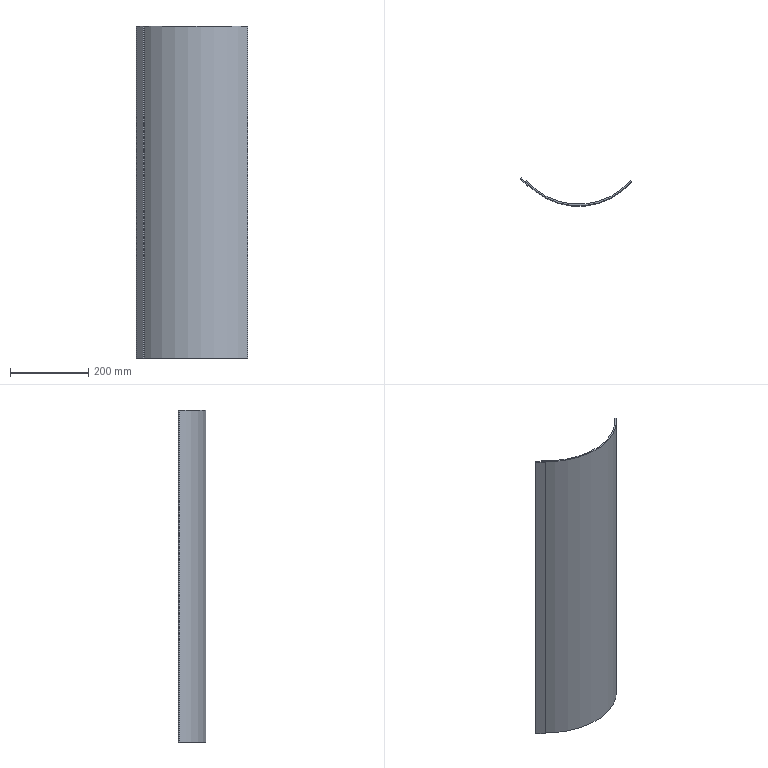Part | SolidWorks | features ExtruThin 1, ICE 1 | 2 solids | 12 faces | box 284.209 x 71.481 x 850 mm | volume 1096694 mm3 | plane 10 | cylinder 2 | commonest cylinder face diameters 354 x1 362 x1
STEP:
#1=CARTESIAN_POINT('',(-135.817,-119.644,-425.));
#2=VERTEX_POINT('',#1);
#3=CARTESIAN_POINT('',(135.817,-119.644,-425.));
#4=VERTEX_POINT('',#3);
#5=CARTESIAN_POINT('',(0.,0.,-425.));
#6=DIRECTION('',(0.,0.,1.));
#7=DIRECTION('',(1.,0.,0.));
#8=AXIS2_PLACEMENT_3D('',#5,#6,#7);
#9=CIRCLE('',#8,181.);
#10=EDGE_CURVE('',#2,#4,#9,.T.);
#11=ORIENTED_EDGE('',*,*,#10,.T.);
#12=CARTESIAN_POINT('',(135.817,-119.644,425.));
#13=VERTEX_POINT('',#12);
#14=CARTESIAN_POINT('',(135.817,-119.644,425.));
#15=DIRECTION('',(0.,0.,-1.));
#16=VECTOR('',#15,1000.);
#17=LINE('',#14,#16);
#18=EDGE_CURVE('',#13,#4,#17,.T.);
#19=ORIENTED_EDGE('',*,*,#18,.F.);
#20=CARTESIAN_POINT('',(-135.817,-119.644,425.));
#21=VERTEX_POINT('',#20);
#22=CARTESIAN_POINT('',(0.,0.,425.));
#23=DIRECTION('',(0.,0.,1.));
#24=DIRECTION('',(1.,0.,0.));
#25=AXIS2_PLACEMENT_3D('',#22,#23,#24);
#26=CIRCLE('',#25,181.);
#27=EDGE_CURVE('',#21,#13,#26,.T.);
#28=ORIENTED_EDGE('',*,*,#27,.F.);
#29=CARTESIAN_POINT('',(-135.817,-119.644,425.));
#30=DIRECTION('',(0.,0.,-1.));
#31=VECTOR('',#30,1000.);
#32=LINE('',#29,#31);
#33=EDGE_CURVE('',#21,#2,#32,.T.);
#34=ORIENTED_EDGE('',*,*,#33,.T.);
#35=EDGE_LOOP('',(#11,#19,#28,#34));
#36=FACE_OUTER_BOUND('',#35,.T.);
#37=CARTESIAN_POINT('',(0.,0.,425.));
#38=DIRECTION('',(0.,0.,-1.));
#39=DIRECTION('',(-1.,0.,0.));
#40=AXIS2_PLACEMENT_3D('',#37,#38,#39);
#41=CYLINDRICAL_SURFACE('',#40,181.);
#42=ADVANCED_FACE('',(#36),#41,.T.);
#43=CARTESIAN_POINT('',(132.816,-117.,-425.));
#44=VERTEX_POINT('',#43);
#45=CARTESIAN_POINT('',(132.816,-117.,-425.));
#46=DIRECTION('',(0.7504,-0.661,0.));
#47=VECTOR('',#46,1000.);
#48=LINE('',#45,#47);
#49=EDGE_CURVE('',#44,#4,#48,.T.);
#50=ORIENTED_EDGE('',*,*,#49,.F.);
#51=CARTESIAN_POINT('',(132.816,-117.,425.));
#52=VERTEX_POINT('',#51);
#53=CARTESIAN_POINT('',(132.816,-117.,425.));
#54=DIRECTION('',(0.,0.,-1.));
#55=VECTOR('',#54,1000.);
#56=LINE('',#53,#55);
#57=EDGE_CURVE('',#52,#44,#56,.T.);
#58=ORIENTED_EDGE('',*,*,#57,.F.);
#59=CARTESIAN_POINT('',(132.816,-117.,425.));
#60=DIRECTION('',(0.7504,-0.661,0.));
#61=VECTOR('',#60,1000.);
#62=LINE('',#59,#61);
#63=EDGE_CURVE('',#52,#13,#62,.T.);
#64=ORIENTED_EDGE('',*,*,#63,.T.);
#65=ORIENTED_EDGE('',*,*,#18,.T.);
#66=EDGE_LOOP('',(#50,#58,#64,#65));
#67=FACE_OUTER_BOUND('',#66,.T.);
#68=CARTESIAN_POINT('',(132.816,-117.,425.));
#69=DIRECTION('',(0.661,0.7504,0.));
#70=DIRECTION('',(-0.7504,0.661,0.));
#71=AXIS2_PLACEMENT_3D('',#68,#69,#70);
#72=PLANE('',#71);
#73=ADVANCED_FACE('',(#67),#72,.T.);
#74=CARTESIAN_POINT('',(-132.816,-117.,-425.));
#75=VERTEX_POINT('',#74);
#76=CARTESIAN_POINT('',(0.,0.,-425.));
#77=DIRECTION('',(0.,0.,1.));
#78=DIRECTION('',(1.,0.,0.));
#79=AXIS2_PLACEMENT_3D('',#76,#77,#78);
#80=CIRCLE('',#79,177.);
#81=EDGE_CURVE('',#75,#44,#80,.T.);
#82=ORIENTED_EDGE('',*,*,#81,.F.);
#83=CARTESIAN_POINT('',(-132.816,-117.,425.));
#84=VERTEX_POINT('',#83);
#85=CARTESIAN_POINT('',(-132.816,-117.,425.));
#86=DIRECTION('',(0.,0.,-1.));
#87=VECTOR('',#86,1000.);
#88=LINE('',#85,#87);
#89=EDGE_CURVE('',#84,#75,#88,.T.);
#90=ORIENTED_EDGE('',*,*,#89,.F.);
#91=CARTESIAN_POINT('',(0.,0.,425.));
#92=DIRECTION('',(0.,0.,1.));
#93=DIRECTION('',(1.,0.,0.));
#94=AXIS2_PLACEMENT_3D('',#91,#92,#93);
#95=CIRCLE('',#94,177.);
#96=EDGE_CURVE('',#84,#52,#95,.T.);
#97=ORIENTED_EDGE('',*,*,#96,.T.);
#98=ORIENTED_EDGE('',*,*,#57,.T.);
#99=EDGE_LOOP('',(#82,#90,#97,#98));
#100=FACE_OUTER_BOUND('',#99,.T.);
#101=CARTESIAN_POINT('',(0.,0.,425.));
#102=DIRECTION('',(0.,0.,-1.));
#103=DIRECTION('',(-1.,0.,0.));
#104=AXIS2_PLACEMENT_3D('',#101,#102,#103);
#105=CYLINDRICAL_SURFACE('',#104,177.);
#106=ADVANCED_FACE('',(#100),#105,.F.);
#107=CARTESIAN_POINT('',(-135.817,-119.644,-425.));
#108=DIRECTION('',(0.7504,0.661,0.));
#109=VECTOR('',#108,1000.);
#110=LINE('',#107,#109);
#111=EDGE_CURVE('',#2,#75,#110,.T.);
#112=ORIENTED_EDGE('',*,*,#111,.F.);
#113=ORIENTED_EDGE('',*,*,#33,.F.);
#114=CARTESIAN_POINT('',(-135.817,-119.644,425.));
#115=DIRECTION('',(0.7504,0.661,0.));
#116=VECTOR('',#115,1000.);
#117=LINE('',#114,#116);
#118=EDGE_CURVE('',#21,#84,#117,.T.);
#119=ORIENTED_EDGE('',*,*,#118,.T.);
#120=ORIENTED_EDGE('',*,*,#89,.T.);
#121=EDGE_LOOP('',(#112,#113,#119,#120));
#122=FACE_OUTER_BOUND('',#121,.T.);
#123=CARTESIAN_POINT('',(-135.817,-119.644,425.));
#124=DIRECTION('',(-0.661,0.7504,0.));
#125=DIRECTION('',(-0.7504,-0.661,0.));
#126=AXIS2_PLACEMENT_3D('',#123,#124,#125);
#127=PLANE('',#126);
#128=ADVANCED_FACE('',(#122),#127,.T.);
#129=ORIENTED_EDGE('',*,*,#27,.T.);
#130=ORIENTED_EDGE('',*,*,#63,.F.);
#131=ORIENTED_EDGE('',*,*,#96,.F.);
#132=ORIENTED_EDGE('',*,*,#118,.F.);
#133=EDGE_LOOP('',(#129,#130,#131,#132));
#134=FACE_OUTER_BOUND('',#133,.T.);
#135=CARTESIAN_POINT('',(0.,0.,425.));
#136=DIRECTION('',(0.,0.,1.));
#137=DIRECTION('',(1.,0.,0.));
#138=AXIS2_PLACEMENT_3D('',#135,#136,#137);
#139=PLANE('',#138);
#140=ADVANCED_FACE('',(#134),#139,.T.);
#141=ORIENTED_EDGE('',*,*,#10,.F.);
#142=ORIENTED_EDGE('',*,*,#111,.T.);
#143=ORIENTED_EDGE('',*,*,#81,.T.);
#144=ORIENTED_EDGE('',*,*,#49,.T.);
#145=EDGE_LOOP('',(#141,#142,#143,#144));
#146=FACE_OUTER_BOUND('',#145,.T.);
#147=CARTESIAN_POINT('',(0.,0.,-425.));
#148=DIRECTION('',(0.,0.,1.));
#149=DIRECTION('',(1.,0.,0.));
#150=AXIS2_PLACEMENT_3D('',#147,#148,#149);
#151=PLANE('',#150);
#152=ADVANCED_FACE('',(#146),#151,.F.);
#153=CLOSED_SHELL('',(#42,#73,#106,#128,#140,#152));
#154=MANIFOLD_SOLID_BREP('',#153);
#155=CARTESIAN_POINT('',(-148.392,-111.628,-425.));
#156=VERTEX_POINT('',#155);
#157=CARTESIAN_POINT('',(-146.259,-109.519,-425.));
#158=VERTEX_POINT('',#157);
#159=CARTESIAN_POINT('',(-148.392,-111.628,-425.));
#160=DIRECTION('',(0.7109,0.7033,0.));
#161=VECTOR('',#160,1000.);
#162=LINE('',#159,#161);
#163=EDGE_CURVE('',#156,#158,#162,.T.);
#164=ORIENTED_EDGE('',*,*,#163,.F.);
#165=CARTESIAN_POINT('',(-148.392,-111.628,425.));
#166=VERTEX_POINT('',#165);
#167=CARTESIAN_POINT('',(-148.392,-111.628,425.));
#168=DIRECTION('',(0.,0.,-1.));
#169=VECTOR('',#168,1000.);
#170=LINE('',#167,#169);
#171=EDGE_CURVE('',#166,#156,#170,.T.);
#172=ORIENTED_EDGE('',*,*,#171,.F.);
#173=CARTESIAN_POINT('',(-146.259,-109.519,425.));
#174=VERTEX_POINT('',#173);
#175=CARTESIAN_POINT('',(-148.392,-111.628,425.));
#176=DIRECTION('',(0.7109,0.7033,0.));
#177=VECTOR('',#176,1000.);
#178=LINE('',#175,#177);
#179=EDGE_CURVE('',#166,#174,#178,.T.);
#180=ORIENTED_EDGE('',*,*,#179,.T.);
#181=CARTESIAN_POINT('',(-146.259,-109.519,425.));
#182=DIRECTION('',(0.,0.,-1.));
#183=VECTOR('',#182,1000.);
#184=LINE('',#181,#183);
#185=EDGE_CURVE('',#174,#158,#184,.T.);
#186=ORIENTED_EDGE('',*,*,#185,.T.);
#187=EDGE_LOOP('',(#164,#172,#180,#186));
#188=FACE_OUTER_BOUND('',#187,.T.);
#189=CARTESIAN_POINT('',(-148.392,-111.628,425.));
#190=DIRECTION('',(-0.7033,0.7109,0.));
#191=DIRECTION('',(-0.7109,-0.7033,0.));
#192=AXIS2_PLACEMENT_3D('',#189,#190,#191);
#193=PLANE('',#192);
#194=ADVANCED_FACE('',(#188),#193,.T.);
#195=CARTESIAN_POINT('',(-130.81,-129.402,-425.));
#196=VERTEX_POINT('',#195);
#197=CARTESIAN_POINT('',(-130.81,-129.402,-425.));
#198=DIRECTION('',(-0.7033,0.7109,0.));
#199=VECTOR('',#198,1000.);
#200=LINE('',#197,#199);
#201=EDGE_CURVE('',#196,#156,#200,.T.);
#202=ORIENTED_EDGE('',*,*,#201,.F.);
#203=CARTESIAN_POINT('',(-130.81,-129.402,425.));
#204=VERTEX_POINT('',#203);
#205=CARTESIAN_POINT('',(-130.81,-129.402,425.));
#206=DIRECTION('',(0.,0.,-1.));
#207=VECTOR('',#206,1000.);
#208=LINE('',#205,#207);
#209=EDGE_CURVE('',#204,#196,#208,.T.);
#210=ORIENTED_EDGE('',*,*,#209,.F.);
#211=CARTESIAN_POINT('',(-130.81,-129.402,425.));
#212=DIRECTION('',(-0.7033,0.7109,0.));
#213=VECTOR('',#212,1000.);
#214=LINE('',#211,#213);
#215=EDGE_CURVE('',#204,#166,#214,.T.);
#216=ORIENTED_EDGE('',*,*,#215,.T.);
#217=ORIENTED_EDGE('',*,*,#171,.T.);
#218=EDGE_LOOP('',(#202,#210,#216,#217));
#219=FACE_OUTER_BOUND('',#218,.T.);
#220=CARTESIAN_POINT('',(-130.81,-129.402,425.));
#221=DIRECTION('',(-0.7109,-0.7033,0.));
#222=DIRECTION('',(0.7033,-0.7109,0.));
#223=AXIS2_PLACEMENT_3D('',#220,#221,#222);
#224=PLANE('',#223);
#225=ADVANCED_FACE('',(#219),#224,.T.);
#226=CARTESIAN_POINT('',(-128.677,-127.292,-425.));
#227=VERTEX_POINT('',#226);
#228=CARTESIAN_POINT('',(-128.677,-127.292,-425.));
#229=DIRECTION('',(-0.7109,-0.7033,0.));
#230=VECTOR('',#229,1000.);
#231=LINE('',#228,#230);
#232=EDGE_CURVE('',#227,#196,#231,.T.);
#233=ORIENTED_EDGE('',*,*,#232,.F.);
#234=CARTESIAN_POINT('',(-128.677,-127.292,425.));
#235=VERTEX_POINT('',#234);
#236=CARTESIAN_POINT('',(-128.677,-127.292,425.));
#237=DIRECTION('',(0.,0.,-1.));
#238=VECTOR('',#237,1000.);
#239=LINE('',#236,#238);
#240=EDGE_CURVE('',#235,#227,#239,.T.);
#241=ORIENTED_EDGE('',*,*,#240,.F.);
#242=CARTESIAN_POINT('',(-128.677,-127.292,425.));
#243=DIRECTION('',(-0.7109,-0.7033,0.));
#244=VECTOR('',#243,1000.);
#245=LINE('',#242,#244);
#246=EDGE_CURVE('',#235,#204,#245,.T.);
#247=ORIENTED_EDGE('',*,*,#246,.T.);
#248=ORIENTED_EDGE('',*,*,#209,.T.);
#249=EDGE_LOOP('',(#233,#241,#247,#248));
#250=FACE_OUTER_BOUND('',#249,.T.);
#251=CARTESIAN_POINT('',(-128.677,-127.292,425.));
#252=DIRECTION('',(0.7033,-0.7109,0.));
#253=DIRECTION('',(0.7109,0.7033,0.));
#254=AXIS2_PLACEMENT_3D('',#251,#252,#253);
#255=PLANE('',#254);
#256=ADVANCED_FACE('',(#250),#255,.T.);
#257=CARTESIAN_POINT('',(-146.259,-109.519,-425.));
#258=DIRECTION('',(0.7033,-0.7109,0.));
#259=VECTOR('',#258,1000.);
#260=LINE('',#257,#259);
#261=EDGE_CURVE('',#158,#227,#260,.T.);
#262=ORIENTED_EDGE('',*,*,#261,.F.);
#263=ORIENTED_EDGE('',*,*,#185,.F.);
#264=CARTESIAN_POINT('',(-146.259,-109.519,425.));
#265=DIRECTION('',(0.7033,-0.7109,0.));
#266=VECTOR('',#265,1000.);
#267=LINE('',#264,#266);
#268=EDGE_CURVE('',#174,#235,#267,.T.);
#269=ORIENTED_EDGE('',*,*,#268,.T.);
#270=ORIENTED_EDGE('',*,*,#240,.T.);
#271=EDGE_LOOP('',(#262,#263,#269,#270));
#272=FACE_OUTER_BOUND('',#271,.T.);
#273=CARTESIAN_POINT('',(-146.259,-109.519,425.));
#274=DIRECTION('',(0.7109,0.7033,0.));
#275=DIRECTION('',(-0.7033,0.7109,0.));
#276=AXIS2_PLACEMENT_3D('',#273,#274,#275);
#277=PLANE('',#276);
#278=ADVANCED_FACE('',(#272),#277,.T.);
#279=ORIENTED_EDGE('',*,*,#179,.F.);
#280=ORIENTED_EDGE('',*,*,#215,.F.);
#281=ORIENTED_EDGE('',*,*,#246,.F.);
#282=ORIENTED_EDGE('',*,*,#268,.F.);
#283=EDGE_LOOP('',(#279,#280,#281,#282));
#284=FACE_OUTER_BOUND('',#283,.T.);
#285=CARTESIAN_POINT('',(0.,0.,425.));
#286=DIRECTION('',(0.,0.,-1.));
#287=DIRECTION('',(-1.,0.,0.));
#288=AXIS2_PLACEMENT_3D('',#285,#286,#287);
#289=PLANE('',#288);
#290=ADVANCED_FACE('',(#284),#289,.F.);
#291=ORIENTED_EDGE('',*,*,#163,.T.);
#292=ORIENTED_EDGE('',*,*,#261,.T.);
#293=ORIENTED_EDGE('',*,*,#232,.T.);
#294=ORIENTED_EDGE('',*,*,#201,.T.);
#295=EDGE_LOOP('',(#291,#292,#293,#294));
#296=FACE_OUTER_BOUND('',#295,.T.);
#297=CARTESIAN_POINT('',(0.,0.,-425.));
#298=DIRECTION('',(0.,0.,-1.));
#299=DIRECTION('',(-1.,0.,0.));
#300=AXIS2_PLACEMENT_3D('',#297,#298,#299);
#301=PLANE('',#300);
#302=ADVANCED_FACE('',(#296),#301,.T.);
#303=CLOSED_SHELL('',(#194,#225,#256,#278,#290,#302));
#304=MANIFOLD_SOLID_BREP('',#303);
#305=CARTESIAN_POINT('',(0.,0.,0.));
#306=DIRECTION('',(0.,0.,1.));
#307=DIRECTION('',(1.,0.,0.));
#308=AXIS2_PLACEMENT_3D('',#305,#306,#307);
#309=(LENGTH_UNIT()NAMED_UNIT(*)SI_UNIT(.MILLI.,.METRE.));
#310=UNCERTAINTY_MEASURE_WITH_UNIT(LENGTH_MEASURE(0.00001),#309,'','');
#311=(NAMED_UNIT(*)PLANE_ANGLE_UNIT()SI_UNIT($,.RADIAN.));
#312=(NAMED_UNIT(*)SI_UNIT($,.STERADIAN.)SOLID_ANGLE_UNIT());
#313=(GEOMETRIC_REPRESENTATION_CONTEXT(3)GLOBAL_UNCERTAINTY_ASSIGNED_CONTEXT((#310))GLOBAL_UNIT_ASSIGNED_CONTEXT((#309,#311,#312))REPRESENTATION_CONTEXT('',''));
#314=ADVANCED_BREP_SHAPE_REPRESENTATION('',(#154,#304,#308),#313);